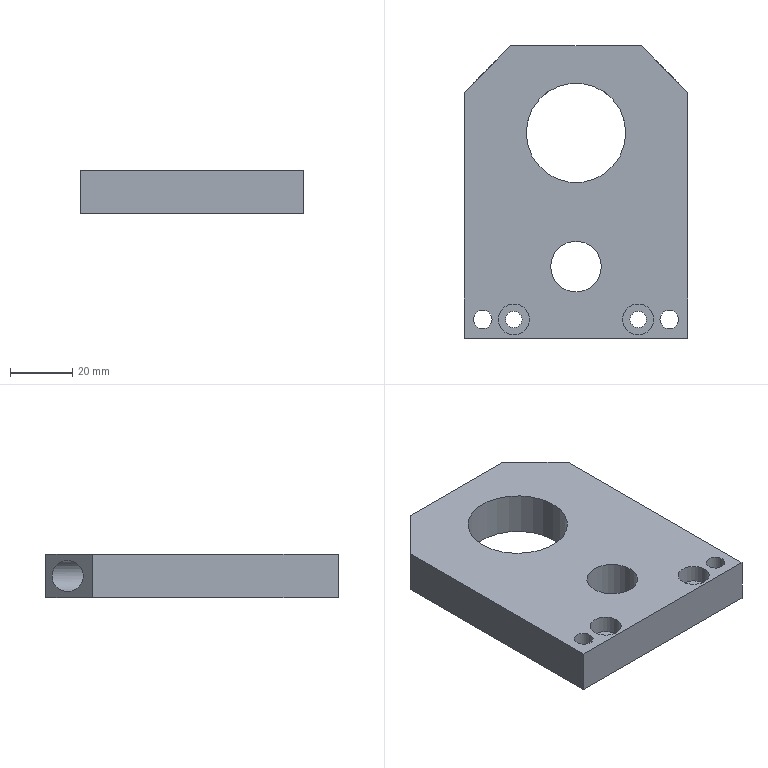Part | NX | 1 solid | 32 faces | box 72 x 94 x 14 mm | volume 72983 mm3 | cylinder 14 | plane 14 | cone 4 | commonest cylinder face diameters 10 x4 4.2 x2 5.3 x2 5.5 x2 6 x2 16.3 x1
STEP:
#1=CARTESIAN_POINT('',(-17.35,-41.,0.));
#2=VERTEX_POINT('',#1);
#3=CARTESIAN_POINT('',(-20.,-41.,0.));
#4=DIRECTION('',(0.,0.,-1.));
#5=DIRECTION('',(1.,0.,0.));
#6=AXIS2_PLACEMENT_3D('',#3,#4,#5);
#7=CIRCLE('',#6,2.65);
#8=EDGE_CURVE('',#2,#2,#7,.T.);
#9=ORIENTED_EDGE('',*,*,#8,.T.);
#10=EDGE_LOOP('',(#9));
#11=FACE_BOUND('',#10,.T.);
#12=CARTESIAN_POINT('',(-17.35,-41.,8.3));
#13=VERTEX_POINT('',#12);
#14=CARTESIAN_POINT('',(-20.,-41.,8.3));
#15=DIRECTION('',(0.,0.,1.));
#16=DIRECTION('',(1.,0.,0.));
#17=AXIS2_PLACEMENT_3D('',#14,#15,#16);
#18=CIRCLE('',#17,2.65);
#19=EDGE_CURVE('',#13,#13,#18,.T.);
#20=ORIENTED_EDGE('',*,*,#19,.T.);
#21=EDGE_LOOP('',(#20));
#22=FACE_BOUND('',#21,.T.);
#23=CARTESIAN_POINT('',(-20.,-41.,0.));
#24=DIRECTION('',(0.,0.,1.));
#25=DIRECTION('',(-1.,0.,0.));
#26=AXIS2_PLACEMENT_3D('',#23,#24,#25);
#27=CYLINDRICAL_SURFACE('',#26,2.65);
#28=ADVANCED_FACE('',(#11,#22),#27,.F.);
#29=CARTESIAN_POINT('',(22.65,-41.,0.));
#30=VERTEX_POINT('',#29);
#31=CARTESIAN_POINT('',(20.,-41.,0.));
#32=DIRECTION('',(0.,0.,-1.));
#33=DIRECTION('',(1.,0.,0.));
#34=AXIS2_PLACEMENT_3D('',#31,#32,#33);
#35=CIRCLE('',#34,2.65);
#36=EDGE_CURVE('',#30,#30,#35,.T.);
#37=ORIENTED_EDGE('',*,*,#36,.T.);
#38=EDGE_LOOP('',(#37));
#39=FACE_BOUND('',#38,.T.);
#40=CARTESIAN_POINT('',(22.65,-41.,8.3));
#41=VERTEX_POINT('',#40);
#42=CARTESIAN_POINT('',(20.,-41.,8.3));
#43=DIRECTION('',(0.,0.,1.));
#44=DIRECTION('',(1.,0.,0.));
#45=AXIS2_PLACEMENT_3D('',#42,#43,#44);
#46=CIRCLE('',#45,2.65);
#47=EDGE_CURVE('',#41,#41,#46,.T.);
#48=ORIENTED_EDGE('',*,*,#47,.T.);
#49=EDGE_LOOP('',(#48));
#50=FACE_BOUND('',#49,.T.);
#51=CARTESIAN_POINT('',(20.,-41.,0.));
#52=DIRECTION('',(0.,0.,1.));
#53=DIRECTION('',(-1.,0.,0.));
#54=AXIS2_PLACEMENT_3D('',#51,#52,#53);
#55=CYLINDRICAL_SURFACE('',#54,2.65);
#56=ADVANCED_FACE('',(#39,#50),#55,.F.);
#57=CARTESIAN_POINT('',(-36.,-47.,14.));
#58=VERTEX_POINT('',#57);
#59=CARTESIAN_POINT('',(-36.,32.,14.));
#60=VERTEX_POINT('',#59);
#61=CARTESIAN_POINT('',(-36.,-47.,14.));
#62=DIRECTION('',(0.,1.,0.));
#63=VECTOR('',#62,1.);
#64=LINE('',#61,#63);
#65=EDGE_CURVE('',#58,#60,#64,.T.);
#66=ORIENTED_EDGE('',*,*,#65,.T.);
#67=CARTESIAN_POINT('',(-36.,32.,0.));
#68=VERTEX_POINT('',#67);
#69=CARTESIAN_POINT('',(-36.,32.,0.));
#70=DIRECTION('',(0.,0.,1.));
#71=VECTOR('',#70,1.);
#72=LINE('',#69,#71);
#73=EDGE_CURVE('',#68,#60,#72,.T.);
#74=ORIENTED_EDGE('',*,*,#73,.F.);
#75=CARTESIAN_POINT('',(-36.,-47.,0.));
#76=VERTEX_POINT('',#75);
#77=CARTESIAN_POINT('',(-36.,-47.,0.));
#78=DIRECTION('',(0.,1.,0.));
#79=VECTOR('',#78,1.);
#80=LINE('',#77,#79);
#81=EDGE_CURVE('',#76,#68,#80,.T.);
#82=ORIENTED_EDGE('',*,*,#81,.F.);
#83=CARTESIAN_POINT('',(-36.,-47.,0.));
#84=DIRECTION('',(0.,0.,1.));
#85=VECTOR('',#84,1.);
#86=LINE('',#83,#85);
#87=EDGE_CURVE('',#76,#58,#86,.T.);
#88=ORIENTED_EDGE('',*,*,#87,.T.);
#89=EDGE_LOOP('',(#66,#74,#82,#88));
#90=FACE_OUTER_BOUND('',#89,.T.);
#91=CARTESIAN_POINT('',(-36.,-47.,0.));
#92=DIRECTION('',(1.,0.,0.));
#93=DIRECTION('',(0.,0.,1.));
#94=AXIS2_PLACEMENT_3D('',#91,#92,#93);
#95=PLANE('',#94);
#96=ADVANCED_FACE('',(#90),#95,.F.);
#97=CARTESIAN_POINT('',(-23.,45.,7.));
#98=VERTEX_POINT('',#97);
#99=CARTESIAN_POINT('',(-28.,40.,7.));
#100=DIRECTION('',(-0.7071,0.7071,0.));
#101=DIRECTION('',(0.7071,0.7071,0.));
#102=AXIS2_PLACEMENT_3D('',#99,#100,#101);
#103=ELLIPSE('',#102,7.071,5.);
#104=EDGE_CURVE('',#98,#98,#103,.T.);
#105=ORIENTED_EDGE('',*,*,#104,.F.);
#106=EDGE_LOOP('',(#105));
#107=FACE_BOUND('',#106,.T.);
#108=CARTESIAN_POINT('',(-21.,47.,14.));
#109=VERTEX_POINT('',#108);
#110=CARTESIAN_POINT('',(-36.,32.,14.));
#111=DIRECTION('',(0.7071,0.7071,0.));
#112=VECTOR('',#111,1.);
#113=LINE('',#110,#112);
#114=EDGE_CURVE('',#60,#109,#113,.T.);
#115=ORIENTED_EDGE('',*,*,#114,.T.);
#116=CARTESIAN_POINT('',(-21.,47.,0.));
#117=VERTEX_POINT('',#116);
#118=CARTESIAN_POINT('',(-21.,47.,0.));
#119=DIRECTION('',(0.,0.,1.));
#120=VECTOR('',#119,1.);
#121=LINE('',#118,#120);
#122=EDGE_CURVE('',#117,#109,#121,.T.);
#123=ORIENTED_EDGE('',*,*,#122,.F.);
#124=CARTESIAN_POINT('',(-36.,32.,0.));
#125=DIRECTION('',(0.7071,0.7071,0.));
#126=VECTOR('',#125,1.);
#127=LINE('',#124,#126);
#128=EDGE_CURVE('',#68,#117,#127,.T.);
#129=ORIENTED_EDGE('',*,*,#128,.F.);
#130=ORIENTED_EDGE('',*,*,#73,.T.);
#131=EDGE_LOOP('',(#115,#123,#129,#130));
#132=FACE_BOUND('',#131,.T.);
#133=CARTESIAN_POINT('',(-36.,32.,0.));
#134=DIRECTION('',(0.7071,-0.7071,0.));
#135=DIRECTION('',(-0.7071,-0.7071,0.));
#136=AXIS2_PLACEMENT_3D('',#133,#134,#135);
#137=PLANE('',#136);
#138=ADVANCED_FACE('',(#107,#132),#137,.F.);
#139=CARTESIAN_POINT('',(21.,47.,14.));
#140=VERTEX_POINT('',#139);
#141=CARTESIAN_POINT('',(-21.,47.,14.));
#142=DIRECTION('',(1.,0.,0.));
#143=VECTOR('',#142,1.);
#144=LINE('',#141,#143);
#145=EDGE_CURVE('',#109,#140,#144,.T.);
#146=ORIENTED_EDGE('',*,*,#145,.T.);
#147=CARTESIAN_POINT('',(21.,47.,0.));
#148=VERTEX_POINT('',#147);
#149=CARTESIAN_POINT('',(21.,47.,0.));
#150=DIRECTION('',(0.,0.,1.));
#151=VECTOR('',#150,1.);
#152=LINE('',#149,#151);
#153=EDGE_CURVE('',#148,#140,#152,.T.);
#154=ORIENTED_EDGE('',*,*,#153,.F.);
#155=CARTESIAN_POINT('',(-21.,47.,0.));
#156=DIRECTION('',(1.,0.,0.));
#157=VECTOR('',#156,1.);
#158=LINE('',#155,#157);
#159=EDGE_CURVE('',#117,#148,#158,.T.);
#160=ORIENTED_EDGE('',*,*,#159,.F.);
#161=ORIENTED_EDGE('',*,*,#122,.T.);
#162=EDGE_LOOP('',(#146,#154,#160,#161));
#163=FACE_OUTER_BOUND('',#162,.T.);
#164=CARTESIAN_POINT('',(-21.,47.,0.));
#165=DIRECTION('',(0.,-1.,0.));
#166=DIRECTION('',(0.,0.,1.));
#167=AXIS2_PLACEMENT_3D('',#164,#165,#166);
#168=PLANE('',#167);
#169=ADVANCED_FACE('',(#163),#168,.F.);
#170=CARTESIAN_POINT('',(23.,45.,7.));
#171=VERTEX_POINT('',#170);
#172=CARTESIAN_POINT('',(28.,40.,7.));
#173=DIRECTION('',(-0.7071,-0.7071,0.));
#174=DIRECTION('',(-0.7071,0.7071,0.));
#175=AXIS2_PLACEMENT_3D('',#172,#173,#174);
#176=ELLIPSE('',#175,7.071,5.);
#177=EDGE_CURVE('',#171,#171,#176,.T.);
#178=ORIENTED_EDGE('',*,*,#177,.T.);
#179=EDGE_LOOP('',(#178));
#180=FACE_BOUND('',#179,.T.);
#181=CARTESIAN_POINT('',(36.,32.,14.));
#182=VERTEX_POINT('',#181);
#183=CARTESIAN_POINT('',(21.,47.,14.));
#184=DIRECTION('',(0.7071,-0.7071,0.));
#185=VECTOR('',#184,1.);
#186=LINE('',#183,#185);
#187=EDGE_CURVE('',#140,#182,#186,.T.);
#188=ORIENTED_EDGE('',*,*,#187,.T.);
#189=CARTESIAN_POINT('',(36.,32.,0.));
#190=VERTEX_POINT('',#189);
#191=CARTESIAN_POINT('',(36.,32.,0.));
#192=DIRECTION('',(0.,0.,1.));
#193=VECTOR('',#192,1.);
#194=LINE('',#191,#193);
#195=EDGE_CURVE('',#190,#182,#194,.T.);
#196=ORIENTED_EDGE('',*,*,#195,.F.);
#197=CARTESIAN_POINT('',(21.,47.,0.));
#198=DIRECTION('',(0.7071,-0.7071,0.));
#199=VECTOR('',#198,1.);
#200=LINE('',#197,#199);
#201=EDGE_CURVE('',#148,#190,#200,.T.);
#202=ORIENTED_EDGE('',*,*,#201,.F.);
#203=ORIENTED_EDGE('',*,*,#153,.T.);
#204=EDGE_LOOP('',(#188,#196,#202,#203));
#205=FACE_BOUND('',#204,.T.);
#206=CARTESIAN_POINT('',(21.,47.,0.));
#207=DIRECTION('',(-0.7071,-0.7071,0.));
#208=DIRECTION('',(-0.7071,0.7071,0.));
#209=AXIS2_PLACEMENT_3D('',#206,#207,#208);
#210=PLANE('',#209);
#211=ADVANCED_FACE('',(#180,#205),#210,.F.);
#212=CARTESIAN_POINT('',(36.,-47.,14.));
#213=VERTEX_POINT('',#212);
#214=CARTESIAN_POINT('',(36.,32.,14.));
#215=DIRECTION('',(0.,-1.,0.));
#216=VECTOR('',#215,1.);
#217=LINE('',#214,#216);
#218=EDGE_CURVE('',#182,#213,#217,.T.);
#219=ORIENTED_EDGE('',*,*,#218,.T.);
#220=CARTESIAN_POINT('',(36.,-47.,0.));
#221=VERTEX_POINT('',#220);
#222=CARTESIAN_POINT('',(36.,-47.,0.));
#223=DIRECTION('',(0.,0.,1.));
#224=VECTOR('',#223,1.);
#225=LINE('',#222,#224);
#226=EDGE_CURVE('',#221,#213,#225,.T.);
#227=ORIENTED_EDGE('',*,*,#226,.F.);
#228=CARTESIAN_POINT('',(36.,32.,0.));
#229=DIRECTION('',(0.,-1.,0.));
#230=VECTOR('',#229,1.);
#231=LINE('',#228,#230);
#232=EDGE_CURVE('',#190,#221,#231,.T.);
#233=ORIENTED_EDGE('',*,*,#232,.F.);
#234=ORIENTED_EDGE('',*,*,#195,.T.);
#235=EDGE_LOOP('',(#219,#227,#233,#234));
#236=FACE_OUTER_BOUND('',#235,.T.);
#237=CARTESIAN_POINT('',(36.,32.,0.));
#238=DIRECTION('',(-1.,0.,0.));
#239=DIRECTION('',(0.,0.,-1.));
#240=AXIS2_PLACEMENT_3D('',#237,#238,#239);
#241=PLANE('',#240);
#242=ADVANCED_FACE('',(#236),#241,.F.);
#243=CARTESIAN_POINT('',(-27.,-41.,14.));
#244=VERTEX_POINT('',#243);
#245=CARTESIAN_POINT('',(-30.,-41.,14.));
#246=DIRECTION('',(0.,0.,1.));
#247=DIRECTION('',(1.,0.,0.));
#248=AXIS2_PLACEMENT_3D('',#245,#246,#247);
#249=CIRCLE('',#248,3.);
#250=EDGE_CURVE('',#244,#244,#249,.T.);
#251=ORIENTED_EDGE('',*,*,#250,.T.);
#252=EDGE_LOOP('',(#251));
#253=FACE_BOUND('',#252,.T.);
#254=CARTESIAN_POINT('',(-27.,-41.,0.));
#255=VERTEX_POINT('',#254);
#256=CARTESIAN_POINT('',(-30.,-41.,0.));
#257=DIRECTION('',(0.,0.,1.));
#258=DIRECTION('',(1.,0.,0.));
#259=AXIS2_PLACEMENT_3D('',#256,#257,#258);
#260=CIRCLE('',#259,3.);
#261=EDGE_CURVE('',#255,#255,#260,.T.);
#262=ORIENTED_EDGE('',*,*,#261,.F.);
#263=EDGE_LOOP('',(#262));
#264=FACE_BOUND('',#263,.T.);
#265=CARTESIAN_POINT('',(-30.,-41.,0.));
#266=DIRECTION('',(0.,0.,1.));
#267=DIRECTION('',(-1.,0.,0.));
#268=AXIS2_PLACEMENT_3D('',#265,#266,#267);
#269=CYLINDRICAL_SURFACE('',#268,3.);
#270=ADVANCED_FACE('',(#253,#264),#269,.F.);
#271=CARTESIAN_POINT('',(16.,19.,14.));
#272=VERTEX_POINT('',#271);
#273=CARTESIAN_POINT('',(0.,19.,14.));
#274=DIRECTION('',(0.,0.,1.));
#275=DIRECTION('',(1.,0.,0.));
#276=AXIS2_PLACEMENT_3D('',#273,#274,#275);
#277=CIRCLE('',#276,16.);
#278=EDGE_CURVE('',#272,#272,#277,.T.);
#279=ORIENTED_EDGE('',*,*,#278,.T.);
#280=EDGE_LOOP('',(#279));
#281=FACE_BOUND('',#280,.T.);
#282=CARTESIAN_POINT('',(16.,19.,0.));
#283=VERTEX_POINT('',#282);
#284=CARTESIAN_POINT('',(0.,19.,0.));
#285=DIRECTION('',(0.,0.,1.));
#286=DIRECTION('',(1.,0.,0.));
#287=AXIS2_PLACEMENT_3D('',#284,#285,#286);
#288=CIRCLE('',#287,16.);
#289=EDGE_CURVE('',#283,#283,#288,.T.);
#290=ORIENTED_EDGE('',*,*,#289,.F.);
#291=EDGE_LOOP('',(#290));
#292=FACE_BOUND('',#291,.T.);
#293=CARTESIAN_POINT('',(0.,19.,0.));
#294=DIRECTION('',(0.,0.,1.));
#295=DIRECTION('',(-1.,0.,0.));
#296=AXIS2_PLACEMENT_3D('',#293,#294,#295);
#297=CYLINDRICAL_SURFACE('',#296,16.);
#298=ADVANCED_FACE('',(#281,#292),#297,.F.);
#299=CARTESIAN_POINT('',(8.15,-24.,14.));
#300=VERTEX_POINT('',#299);
#301=CARTESIAN_POINT('',(0.,-24.,14.));
#302=DIRECTION('',(0.,0.,1.));
#303=DIRECTION('',(1.,0.,0.));
#304=AXIS2_PLACEMENT_3D('',#301,#302,#303);
#305=CIRCLE('',#304,8.15);
#306=EDGE_CURVE('',#300,#300,#305,.T.);
#307=ORIENTED_EDGE('',*,*,#306,.T.);
#308=EDGE_LOOP('',(#307));
#309=FACE_BOUND('',#308,.T.);
#310=CARTESIAN_POINT('',(8.15,-24.,0.));
#311=VERTEX_POINT('',#310);
#312=CARTESIAN_POINT('',(0.,-24.,0.));
#313=DIRECTION('',(0.,0.,1.));
#314=DIRECTION('',(1.,0.,0.));
#315=AXIS2_PLACEMENT_3D('',#312,#313,#314);
#316=CIRCLE('',#315,8.15);
#317=EDGE_CURVE('',#311,#311,#316,.T.);
#318=ORIENTED_EDGE('',*,*,#317,.F.);
#319=EDGE_LOOP('',(#318));
#320=FACE_BOUND('',#319,.T.);
#321=CARTESIAN_POINT('',(0.,-24.,0.));
#322=DIRECTION('',(0.,0.,1.));
#323=DIRECTION('',(-1.,0.,0.));
#324=AXIS2_PLACEMENT_3D('',#321,#322,#323);
#325=CYLINDRICAL_SURFACE('',#324,8.15);
#326=ADVANCED_FACE('',(#309,#320),#325,.F.);
#327=CARTESIAN_POINT('',(33.,-41.,14.));
#328=VERTEX_POINT('',#327);
#329=CARTESIAN_POINT('',(30.,-41.,14.));
#330=DIRECTION('',(0.,0.,1.));
#331=DIRECTION('',(1.,0.,0.));
#332=AXIS2_PLACEMENT_3D('',#329,#330,#331);
#333=CIRCLE('',#332,3.);
#334=EDGE_CURVE('',#328,#328,#333,.T.);
#335=ORIENTED_EDGE('',*,*,#334,.T.);
#336=EDGE_LOOP('',(#335));
#337=FACE_BOUND('',#336,.T.);
#338=CARTESIAN_POINT('',(33.,-41.,0.));
#339=VERTEX_POINT('',#338);
#340=CARTESIAN_POINT('',(30.,-41.,0.));
#341=DIRECTION('',(0.,0.,1.));
#342=DIRECTION('',(1.,0.,0.));
#343=AXIS2_PLACEMENT_3D('',#340,#341,#342);
#344=CIRCLE('',#343,3.);
#345=EDGE_CURVE('',#339,#339,#344,.T.);
#346=ORIENTED_EDGE('',*,*,#345,.F.);
#347=EDGE_LOOP('',(#346));
#348=FACE_BOUND('',#347,.T.);
#349=CARTESIAN_POINT('',(30.,-41.,0.));
#350=DIRECTION('',(0.,0.,1.));
#351=DIRECTION('',(-1.,0.,0.));
#352=AXIS2_PLACEMENT_3D('',#349,#350,#351);
#353=CYLINDRICAL_SURFACE('',#352,3.);
#354=ADVANCED_FACE('',(#337,#348),#353,.F.);
#355=CARTESIAN_POINT('',(36.,-47.,14.));
#356=DIRECTION('',(-1.,0.,0.));
#357=VECTOR('',#356,1.);
#358=LINE('',#355,#357);
#359=EDGE_CURVE('',#213,#58,#358,.T.);
#360=ORIENTED_EDGE('',*,*,#359,.T.);
#361=ORIENTED_EDGE('',*,*,#87,.F.);
#362=CARTESIAN_POINT('',(36.,-47.,0.));
#363=DIRECTION('',(-1.,0.,0.));
#364=VECTOR('',#363,1.);
#365=LINE('',#362,#364);
#366=EDGE_CURVE('',#221,#76,#365,.T.);
#367=ORIENTED_EDGE('',*,*,#366,.F.);
#368=ORIENTED_EDGE('',*,*,#226,.T.);
#369=EDGE_LOOP('',(#360,#361,#367,#368));
#370=FACE_OUTER_BOUND('',#369,.T.);
#371=CARTESIAN_POINT('',(36.,-47.,0.));
#372=DIRECTION('',(0.,1.,0.));
#373=DIRECTION('',(0.,0.,-1.));
#374=AXIS2_PLACEMENT_3D('',#371,#372,#373);
#375=PLANE('',#374);
#376=ADVANCED_FACE('',(#370),#375,.F.);
#377=ORIENTED_EDGE('',*,*,#81,.T.);
#378=ORIENTED_EDGE('',*,*,#128,.T.);
#379=ORIENTED_EDGE('',*,*,#159,.T.);
#380=ORIENTED_EDGE('',*,*,#201,.T.);
#381=ORIENTED_EDGE('',*,*,#232,.T.);
#382=ORIENTED_EDGE('',*,*,#366,.T.);
#383=EDGE_LOOP('',(#377,#378,#379,#380,#381,#382));
#384=FACE_BOUND('',#383,.T.);
#385=ORIENTED_EDGE('',*,*,#345,.T.);
#386=EDGE_LOOP('',(#385));
#387=FACE_BOUND('',#386,.T.);
#388=ORIENTED_EDGE('',*,*,#317,.T.);
#389=EDGE_LOOP('',(#388));
#390=FACE_BOUND('',#389,.T.);
#391=ORIENTED_EDGE('',*,*,#289,.T.);
#392=EDGE_LOOP('',(#391));
#393=FACE_BOUND('',#392,.T.);
#394=ORIENTED_EDGE('',*,*,#261,.T.);
#395=EDGE_LOOP('',(#394));
#396=FACE_BOUND('',#395,.T.);
#397=ORIENTED_EDGE('',*,*,#8,.F.);
#398=EDGE_LOOP('',(#397));
#399=FACE_BOUND('',#398,.T.);
#400=ORIENTED_EDGE('',*,*,#36,.F.);
#401=EDGE_LOOP('',(#400));
#402=FACE_BOUND('',#401,.T.);
#403=CARTESIAN_POINT('',(30.,-41.,0.));
#404=DIRECTION('',(0.,0.,1.));
#405=DIRECTION('',(-1.,0.,0.));
#406=AXIS2_PLACEMENT_3D('',#403,#404,#405);
#407=PLANE('',#406);
#408=ADVANCED_FACE('',(#384,#387,#390,#393,#396,#399,#402),#407,.F.);
#409=CARTESIAN_POINT('',(25.,-41.,14.));
#410=VERTEX_POINT('',#409);
#411=CARTESIAN_POINT('',(20.,-41.,14.));
#412=DIRECTION('',(0.,0.,1.));
#413=DIRECTION('',(1.,0.,0.));
#414=AXIS2_PLACEMENT_3D('',#411,#412,#413);
#415=CIRCLE('',#414,5.);
#416=EDGE_CURVE('',#410,#410,#415,.T.);
#417=ORIENTED_EDGE('',*,*,#416,.F.);
#418=EDGE_LOOP('',(#417));
#419=FACE_BOUND('',#418,.T.);
#420=CARTESIAN_POINT('',(-15.,-41.,14.));
#421=VERTEX_POINT('',#420);
#422=CARTESIAN_POINT('',(-20.,-41.,14.));
#423=DIRECTION('',(0.,0.,1.));
#424=DIRECTION('',(1.,0.,0.));
#425=AXIS2_PLACEMENT_3D('',#422,#423,#424);
#426=CIRCLE('',#425,5.);
#427=EDGE_CURVE('',#421,#421,#426,.T.);
#428=ORIENTED_EDGE('',*,*,#427,.F.);
#429=EDGE_LOOP('',(#428));
#430=FACE_BOUND('',#429,.T.);
#431=ORIENTED_EDGE('',*,*,#65,.F.);
#432=ORIENTED_EDGE('',*,*,#359,.F.);
#433=ORIENTED_EDGE('',*,*,#218,.F.);
#434=ORIENTED_EDGE('',*,*,#187,.F.);
#435=ORIENTED_EDGE('',*,*,#145,.F.);
#436=ORIENTED_EDGE('',*,*,#114,.F.);
#437=EDGE_LOOP('',(#431,#432,#433,#434,#435,#436));
#438=FACE_BOUND('',#437,.T.);
#439=ORIENTED_EDGE('',*,*,#334,.F.);
#440=EDGE_LOOP('',(#439));
#441=FACE_BOUND('',#440,.T.);
#442=ORIENTED_EDGE('',*,*,#306,.F.);
#443=EDGE_LOOP('',(#442));
#444=FACE_BOUND('',#443,.T.);
#445=ORIENTED_EDGE('',*,*,#278,.F.);
#446=EDGE_LOOP('',(#445));
#447=FACE_BOUND('',#446,.T.);
#448=ORIENTED_EDGE('',*,*,#250,.F.);
#449=EDGE_LOOP('',(#448));
#450=FACE_BOUND('',#449,.T.);
#451=CARTESIAN_POINT('',(30.,-41.,14.));
#452=DIRECTION('',(0.,0.,1.));
#453=DIRECTION('',(-1.,0.,0.));
#454=AXIS2_PLACEMENT_3D('',#451,#452,#453);
#455=PLANE('',#454);
#456=ADVANCED_FACE('',(#419,#430,#438,#441,#444,#447,#450),#455,.T.);
#457=ORIENTED_EDGE('',*,*,#427,.T.);
#458=EDGE_LOOP('',(#457));
#459=FACE_BOUND('',#458,.T.);
#460=CARTESIAN_POINT('',(-15.,-41.,8.3));
#461=VERTEX_POINT('',#460);
#462=CARTESIAN_POINT('',(-20.,-41.,8.3));
#463=DIRECTION('',(0.,0.,-1.));
#464=DIRECTION('',(1.,0.,0.));
#465=AXIS2_PLACEMENT_3D('',#462,#463,#464);
#466=CIRCLE('',#465,5.);
#467=EDGE_CURVE('',#461,#461,#466,.T.);
#468=ORIENTED_EDGE('',*,*,#467,.T.);
#469=EDGE_LOOP('',(#468));
#470=FACE_BOUND('',#469,.T.);
#471=CARTESIAN_POINT('',(-20.,-41.,8.3));
#472=DIRECTION('',(0.,0.,1.));
#473=DIRECTION('',(-1.,0.,0.));
#474=AXIS2_PLACEMENT_3D('',#471,#472,#473);
#475=CYLINDRICAL_SURFACE('',#474,5.);
#476=ADVANCED_FACE('',(#459,#470),#475,.F.);
#477=ORIENTED_EDGE('',*,*,#19,.F.);
#478=EDGE_LOOP('',(#477));
#479=FACE_BOUND('',#478,.T.);
#480=ORIENTED_EDGE('',*,*,#467,.F.);
#481=EDGE_LOOP('',(#480));
#482=FACE_BOUND('',#481,.T.);
#483=CARTESIAN_POINT('',(-20.,-41.,8.3));
#484=DIRECTION('',(0.,0.,1.));
#485=DIRECTION('',(-1.,0.,0.));
#486=AXIS2_PLACEMENT_3D('',#483,#484,#485);
#487=PLANE('',#486);
#488=ADVANCED_FACE('',(#479,#482),#487,.T.);
#489=ORIENTED_EDGE('',*,*,#416,.T.);
#490=EDGE_LOOP('',(#489));
#491=FACE_BOUND('',#490,.T.);
#492=CARTESIAN_POINT('',(25.,-41.,8.3));
#493=VERTEX_POINT('',#492);
#494=CARTESIAN_POINT('',(20.,-41.,8.3));
#495=DIRECTION('',(0.,0.,-1.));
#496=DIRECTION('',(1.,0.,0.));
#497=AXIS2_PLACEMENT_3D('',#494,#495,#496);
#498=CIRCLE('',#497,5.);
#499=EDGE_CURVE('',#493,#493,#498,.T.);
#500=ORIENTED_EDGE('',*,*,#499,.T.);
#501=EDGE_LOOP('',(#500));
#502=FACE_BOUND('',#501,.T.);
#503=CARTESIAN_POINT('',(20.,-41.,8.3));
#504=DIRECTION('',(0.,0.,1.));
#505=DIRECTION('',(-1.,0.,0.));
#506=AXIS2_PLACEMENT_3D('',#503,#504,#505);
#507=CYLINDRICAL_SURFACE('',#506,5.);
#508=ADVANCED_FACE('',(#491,#502),#507,.F.);
#509=ORIENTED_EDGE('',*,*,#47,.F.);
#510=EDGE_LOOP('',(#509));
#511=FACE_BOUND('',#510,.T.);
#512=ORIENTED_EDGE('',*,*,#499,.F.);
#513=EDGE_LOOP('',(#512));
#514=FACE_BOUND('',#513,.T.);
#515=CARTESIAN_POINT('',(20.,-41.,8.3));
#516=DIRECTION('',(0.,0.,1.));
#517=DIRECTION('',(-1.,0.,0.));
#518=AXIS2_PLACEMENT_3D('',#515,#516,#517);
#519=PLANE('',#518);
#520=ADVANCED_FACE('',(#511,#514),#519,.T.);
#521=CARTESIAN_POINT('',(-28.,30.,12.));
#522=VERTEX_POINT('',#521);
#523=CARTESIAN_POINT('',(-28.,30.,7.));
#524=DIRECTION('',(0.,1.,0.));
#525=DIRECTION('',(0.,0.,1.));
#526=AXIS2_PLACEMENT_3D('',#523,#524,#525);
#527=CIRCLE('',#526,5.);
#528=EDGE_CURVE('',#522,#522,#527,.T.);
#529=ORIENTED_EDGE('',*,*,#528,.F.);
#530=EDGE_LOOP('',(#529));
#531=FACE_BOUND('',#530,.T.);
#532=ORIENTED_EDGE('',*,*,#104,.T.);
#533=EDGE_LOOP('',(#532));
#534=FACE_BOUND('',#533,.T.);
#535=CARTESIAN_POINT('',(-28.,30.,7.));
#536=DIRECTION('',(0.,1.,0.));
#537=DIRECTION('',(0.,0.,-1.));
#538=AXIS2_PLACEMENT_3D('',#535,#536,#537);
#539=CYLINDRICAL_SURFACE('',#538,5.);
#540=ADVANCED_FACE('',(#531,#534),#539,.F.);
#541=CARTESIAN_POINT('',(-28.,30.,4.25));
#542=VERTEX_POINT('',#541);
#543=CARTESIAN_POINT('',(-28.,30.,7.));
#544=DIRECTION('',(0.,-1.,0.));
#545=DIRECTION('',(0.,0.,-1.));
#546=AXIS2_PLACEMENT_3D('',#543,#544,#545);
#547=CIRCLE('',#546,2.75);
#548=EDGE_CURVE('',#542,#542,#547,.T.);
#549=ORIENTED_EDGE('',*,*,#548,.T.);
#550=EDGE_LOOP('',(#549));
#551=FACE_BOUND('',#550,.T.);
#552=ORIENTED_EDGE('',*,*,#528,.T.);
#553=EDGE_LOOP('',(#552));
#554=FACE_BOUND('',#553,.T.);
#555=CARTESIAN_POINT('',(-28.,30.,7.));
#556=DIRECTION('',(0.,-1.,0.));
#557=DIRECTION('',(0.,0.,1.));
#558=AXIS2_PLACEMENT_3D('',#555,#556,#557);
#559=PLANE('',#558);
#560=ADVANCED_FACE('',(#551,#554),#559,.F.);
#561=CARTESIAN_POINT('',(28.,30.,12.));
#562=VERTEX_POINT('',#561);
#563=CARTESIAN_POINT('',(28.,30.,7.));
#564=DIRECTION('',(0.,-1.,0.));
#565=DIRECTION('',(0.,0.,1.));
#566=AXIS2_PLACEMENT_3D('',#563,#564,#565);
#567=CIRCLE('',#566,5.);
#568=EDGE_CURVE('',#562,#562,#567,.T.);
#569=ORIENTED_EDGE('',*,*,#568,.T.);
#570=EDGE_LOOP('',(#569));
#571=FACE_BOUND('',#570,.T.);
#572=ORIENTED_EDGE('',*,*,#177,.F.);
#573=EDGE_LOOP('',(#572));
#574=FACE_BOUND('',#573,.T.);
#575=CARTESIAN_POINT('',(28.,30.,7.));
#576=DIRECTION('',(0.,1.,0.));
#577=DIRECTION('',(0.,0.,-1.));
#578=AXIS2_PLACEMENT_3D('',#575,#576,#577);
#579=CYLINDRICAL_SURFACE('',#578,5.);
#580=ADVANCED_FACE('',(#571,#574),#579,.F.);
#581=CARTESIAN_POINT('',(28.,30.,9.75));
#582=VERTEX_POINT('',#581);
#583=CARTESIAN_POINT('',(28.,30.,7.));
#584=DIRECTION('',(0.,1.,0.));
#585=DIRECTION('',(0.,0.,1.));
#586=AXIS2_PLACEMENT_3D('',#583,#584,#585);
#587=CIRCLE('',#586,2.75);
#588=EDGE_CURVE('',#582,#582,#587,.T.);
#589=ORIENTED_EDGE('',*,*,#588,.F.);
#590=EDGE_LOOP('',(#589));
#591=FACE_BOUND('',#590,.T.);
#592=ORIENTED_EDGE('',*,*,#568,.F.);
#593=EDGE_LOOP('',(#592));
#594=FACE_BOUND('',#593,.T.);
#595=CARTESIAN_POINT('',(28.,30.,7.));
#596=DIRECTION('',(0.,1.,0.));
#597=DIRECTION('',(0.,0.,-1.));
#598=AXIS2_PLACEMENT_3D('',#595,#596,#597);
#599=PLANE('',#598);
#600=ADVANCED_FACE('',(#591,#594),#599,.T.);
#601=CARTESIAN_POINT('',(-28.,19.,4.5));
#602=VERTEX_POINT('',#601);
#603=CARTESIAN_POINT('',(-28.,19.,7.));
#604=DIRECTION('',(0.,-1.,0.));
#605=DIRECTION('',(0.,0.,-1.));
#606=AXIS2_PLACEMENT_3D('',#603,#604,#605);
#607=CIRCLE('',#606,2.5);
#608=EDGE_CURVE('',#602,#602,#607,.T.);
#609=ORIENTED_EDGE('',*,*,#608,.T.);
#610=EDGE_LOOP('',(#609));
#611=FACE_BOUND('',#610,.T.);
#612=CARTESIAN_POINT('',(-28.,19.,9.75));
#613=VERTEX_POINT('',#612);
#614=CARTESIAN_POINT('',(-28.,19.,7.));
#615=DIRECTION('',(0.,1.,0.));
#616=DIRECTION('',(0.,0.,1.));
#617=AXIS2_PLACEMENT_3D('',#614,#615,#616);
#618=CIRCLE('',#617,2.75);
#619=EDGE_CURVE('',#613,#613,#618,.T.);
#620=ORIENTED_EDGE('',*,*,#619,.T.);
#621=EDGE_LOOP('',(#620));
#622=FACE_BOUND('',#621,.T.);
#623=CARTESIAN_POINT('',(-28.,19.,7.));
#624=DIRECTION('',(0.,-1.,0.));
#625=DIRECTION('',(0.,0.,1.));
#626=AXIS2_PLACEMENT_3D('',#623,#624,#625);
#627=PLANE('',#626);
#628=ADVANCED_FACE('',(#611,#622),#627,.F.);
#629=ORIENTED_EDGE('',*,*,#548,.F.);
#630=EDGE_LOOP('',(#629));
#631=FACE_BOUND('',#630,.T.);
#632=ORIENTED_EDGE('',*,*,#619,.F.);
#633=EDGE_LOOP('',(#632));
#634=FACE_BOUND('',#633,.T.);
#635=CARTESIAN_POINT('',(-28.,19.,7.));
#636=DIRECTION('',(0.,1.,0.));
#637=DIRECTION('',(0.,0.,-1.));
#638=AXIS2_PLACEMENT_3D('',#635,#636,#637);
#639=CYLINDRICAL_SURFACE('',#638,2.75);
#640=ADVANCED_FACE('',(#631,#634),#639,.F.);
#641=CARTESIAN_POINT('',(28.,19.,4.5));
#642=VERTEX_POINT('',#641);
#643=CARTESIAN_POINT('',(28.,19.,7.));
#644=DIRECTION('',(0.,-1.,0.));
#645=DIRECTION('',(0.,0.,-1.));
#646=AXIS2_PLACEMENT_3D('',#643,#644,#645);
#647=CIRCLE('',#646,2.5);
#648=EDGE_CURVE('',#642,#642,#647,.T.);
#649=ORIENTED_EDGE('',*,*,#648,.T.);
#650=EDGE_LOOP('',(#649));
#651=FACE_BOUND('',#650,.T.);
#652=CARTESIAN_POINT('',(28.,19.,9.75));
#653=VERTEX_POINT('',#652);
#654=CARTESIAN_POINT('',(28.,19.,7.));
#655=DIRECTION('',(0.,1.,0.));
#656=DIRECTION('',(0.,0.,1.));
#657=AXIS2_PLACEMENT_3D('',#654,#655,#656);
#658=CIRCLE('',#657,2.75);
#659=EDGE_CURVE('',#653,#653,#658,.T.);
#660=ORIENTED_EDGE('',*,*,#659,.T.);
#661=EDGE_LOOP('',(#660));
#662=FACE_BOUND('',#661,.T.);
#663=CARTESIAN_POINT('',(28.,19.,7.));
#664=DIRECTION('',(0.,-1.,0.));
#665=DIRECTION('',(0.,0.,1.));
#666=AXIS2_PLACEMENT_3D('',#663,#664,#665);
#667=PLANE('',#666);
#668=ADVANCED_FACE('',(#651,#662),#667,.F.);
#669=ORIENTED_EDGE('',*,*,#659,.F.);
#670=EDGE_LOOP('',(#669));
#671=FACE_BOUND('',#670,.T.);
#672=ORIENTED_EDGE('',*,*,#588,.T.);
#673=EDGE_LOOP('',(#672));
#674=FACE_BOUND('',#673,.T.);
#675=CARTESIAN_POINT('',(28.,19.,7.));
#676=DIRECTION('',(0.,1.,0.));
#677=DIRECTION('',(0.,0.,-1.));
#678=AXIS2_PLACEMENT_3D('',#675,#676,#677);
#679=CYLINDRICAL_SURFACE('',#678,2.75);
#680=ADVANCED_FACE('',(#671,#674),#679,.F.);
#681=CARTESIAN_POINT('',(-28.,9.,4.9));
#682=VERTEX_POINT('',#681);
#683=CARTESIAN_POINT('',(-28.,9.,7.));
#684=DIRECTION('',(0.,1.,0.));
#685=DIRECTION('',(0.,0.,-1.));
#686=AXIS2_PLACEMENT_3D('',#683,#684,#685);
#687=CIRCLE('',#686,2.1);
#688=EDGE_CURVE('',#682,#682,#687,.T.);
#689=ORIENTED_EDGE('',*,*,#688,.T.);
#690=EDGE_LOOP('',(#689));
#691=FACE_BOUND('',#690,.T.);
#692=CARTESIAN_POINT('',(-28.,7.738,7.));
#693=VERTEX_POINT('',#692);
#694=VERTEX_LOOP('',#693);
#695=FACE_BOUND('',#694,.T.);
#696=CARTESIAN_POINT('',(-28.,9.,7.));
#697=DIRECTION('',(0.,1.,0.));
#698=DIRECTION('',(0.,0.,-1.));
#699=AXIS2_PLACEMENT_3D('',#696,#697,#698);
#700=CONICAL_SURFACE('',#699,2.1,59.);
#701=ADVANCED_FACE('',(#691,#695),#700,.F.);
#702=CARTESIAN_POINT('',(-28.,18.6,4.9));
#703=VERTEX_POINT('',#702);
#704=CARTESIAN_POINT('',(-28.,18.6,7.));
#705=DIRECTION('',(0.,1.,0.));
#706=DIRECTION('',(0.,0.,-1.));
#707=AXIS2_PLACEMENT_3D('',#704,#705,#706);
#708=CIRCLE('',#707,2.1);
#709=EDGE_CURVE('',#703,#703,#708,.T.);
#710=ORIENTED_EDGE('',*,*,#709,.T.);
#711=EDGE_LOOP('',(#710));
#712=FACE_BOUND('',#711,.T.);
#713=ORIENTED_EDGE('',*,*,#688,.F.);
#714=EDGE_LOOP('',(#713));
#715=FACE_BOUND('',#714,.T.);
#716=CARTESIAN_POINT('',(-28.,19.,7.));
#717=DIRECTION('',(0.,-1.,0.));
#718=DIRECTION('',(0.,0.,1.));
#719=AXIS2_PLACEMENT_3D('',#716,#717,#718);
#720=CYLINDRICAL_SURFACE('',#719,2.1);
#721=ADVANCED_FACE('',(#712,#715),#720,.F.);
#722=ORIENTED_EDGE('',*,*,#709,.F.);
#723=EDGE_LOOP('',(#722));
#724=FACE_BOUND('',#723,.T.);
#725=ORIENTED_EDGE('',*,*,#608,.F.);
#726=EDGE_LOOP('',(#725));
#727=FACE_BOUND('',#726,.T.);
#728=CARTESIAN_POINT('',(-28.,19.,7.));
#729=DIRECTION('',(0.,1.,0.));
#730=DIRECTION('',(0.,0.,-1.));
#731=AXIS2_PLACEMENT_3D('',#728,#729,#730);
#732=CONICAL_SURFACE('',#731,2.5,45.);
#733=ADVANCED_FACE('',(#724,#727),#732,.F.);
#734=CARTESIAN_POINT('',(28.,9.,4.9));
#735=VERTEX_POINT('',#734);
#736=CARTESIAN_POINT('',(28.,9.,7.));
#737=DIRECTION('',(0.,1.,0.));
#738=DIRECTION('',(0.,0.,-1.));
#739=AXIS2_PLACEMENT_3D('',#736,#737,#738);
#740=CIRCLE('',#739,2.1);
#741=EDGE_CURVE('',#735,#735,#740,.T.);
#742=ORIENTED_EDGE('',*,*,#741,.T.);
#743=EDGE_LOOP('',(#742));
#744=FACE_BOUND('',#743,.T.);
#745=CARTESIAN_POINT('',(28.,7.738,7.));
#746=VERTEX_POINT('',#745);
#747=VERTEX_LOOP('',#746);
#748=FACE_BOUND('',#747,.T.);
#749=CARTESIAN_POINT('',(28.,9.,7.));
#750=DIRECTION('',(0.,1.,0.));
#751=DIRECTION('',(0.,0.,-1.));
#752=AXIS2_PLACEMENT_3D('',#749,#750,#751);
#753=CONICAL_SURFACE('',#752,2.1,59.);
#754=ADVANCED_FACE('',(#744,#748),#753,.F.);
#755=CARTESIAN_POINT('',(28.,18.6,4.9));
#756=VERTEX_POINT('',#755);
#757=CARTESIAN_POINT('',(28.,18.6,7.));
#758=DIRECTION('',(0.,1.,0.));
#759=DIRECTION('',(0.,0.,-1.));
#760=AXIS2_PLACEMENT_3D('',#757,#758,#759);
#761=CIRCLE('',#760,2.1);
#762=EDGE_CURVE('',#756,#756,#761,.T.);
#763=ORIENTED_EDGE('',*,*,#762,.T.);
#764=EDGE_LOOP('',(#763));
#765=FACE_BOUND('',#764,.T.);
#766=ORIENTED_EDGE('',*,*,#741,.F.);
#767=EDGE_LOOP('',(#766));
#768=FACE_BOUND('',#767,.T.);
#769=CARTESIAN_POINT('',(28.,19.,7.));
#770=DIRECTION('',(0.,-1.,0.));
#771=DIRECTION('',(0.,0.,1.));
#772=AXIS2_PLACEMENT_3D('',#769,#770,#771);
#773=CYLINDRICAL_SURFACE('',#772,2.1);
#774=ADVANCED_FACE('',(#765,#768),#773,.F.);
#775=ORIENTED_EDGE('',*,*,#762,.F.);
#776=EDGE_LOOP('',(#775));
#777=FACE_BOUND('',#776,.T.);
#778=ORIENTED_EDGE('',*,*,#648,.F.);
#779=EDGE_LOOP('',(#778));
#780=FACE_BOUND('',#779,.T.);
#781=CARTESIAN_POINT('',(28.,19.,7.));
#782=DIRECTION('',(0.,1.,0.));
#783=DIRECTION('',(0.,0.,-1.));
#784=AXIS2_PLACEMENT_3D('',#781,#782,#783);
#785=CONICAL_SURFACE('',#784,2.5,45.);
#786=ADVANCED_FACE('',(#777,#780),#785,.F.);
#787=CLOSED_SHELL('',(#28,#56,#96,#138,#169,#211,#242,#270,#298,#326,#354,#376,#408,#456,#476,#488,#508,#520,#540,#560,#580,#600,#628,#640,#668,#680,#701,#721,#733,#754,#774,#786));
#788=MANIFOLD_SOLID_BREP('',#787);
#789=(LENGTH_UNIT()NAMED_UNIT(*)SI_UNIT(.MILLI.,.METRE.));
#790=UNCERTAINTY_MEASURE_WITH_UNIT(LENGTH_MEASURE(0.00002),#789,'','');
#791=(NAMED_UNIT(*)PLANE_ANGLE_UNIT()SI_UNIT($,.RADIAN.));
#792=PLANE_ANGLE_MEASURE_WITH_UNIT(PLANE_ANGLE_MEASURE(0.01745),#791);
#793=DIMENSIONAL_EXPONENTS(0.,0.,0.,0.,0.,0.,0.);
#794=(CONVERSION_BASED_UNIT('DEGREE',#792)NAMED_UNIT(#793)PLANE_ANGLE_UNIT());
#795=(NAMED_UNIT(*)SI_UNIT($,.STERADIAN.)SOLID_ANGLE_UNIT());
#796=(GEOMETRIC_REPRESENTATION_CONTEXT(3)GLOBAL_UNCERTAINTY_ASSIGNED_CONTEXT((#790))GLOBAL_UNIT_ASSIGNED_CONTEXT((#789,#794,#795))REPRESENTATION_CONTEXT('',''));
#797=ADVANCED_BREP_SHAPE_REPRESENTATION('',(#788),#796);